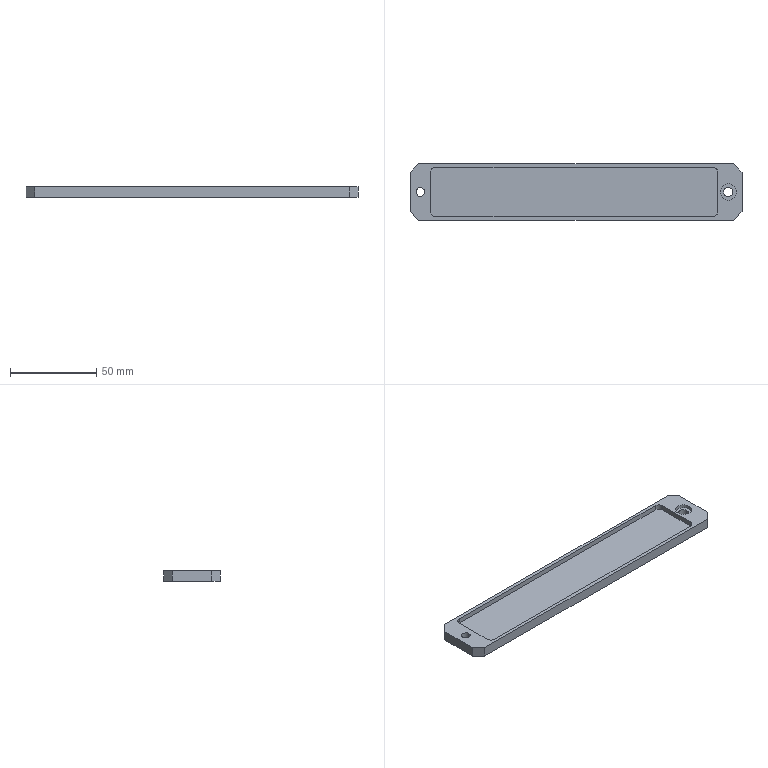Part | STEP file | J454-EBZ05-34-00-Part-1-3 | 1 solid | 26 faces | box 193 x 33 x 6 mm | volume 23054 mm3 | plane 16 | cylinder 10 | commonest cylinder face diameters 6 x4 5 x2 5.5 x2 9.5 x2
STEP:
#1=CARTESIAN_POINT('',(181.75,0.,0.));
#2=VERTEX_POINT('',#1);
#3=CARTESIAN_POINT('',(176.25,0.,0.));
#4=VERTEX_POINT('',#3);
#5=CARTESIAN_POINT('',(179.,0.,0.));
#6=DIRECTION('',(0.,0.,1.));
#7=DIRECTION('',(-1.,0.,0.));
#8=AXIS2_PLACEMENT_3D('',#5,#6,#7);
#9=CIRCLE('',#8,2.75);
#10=EDGE_CURVE('',#2,#4,#9,.T.);
#11=ORIENTED_EDGE('',*,*,#10,.F.);
#12=CARTESIAN_POINT('',(181.75,0.,4.));
#13=VERTEX_POINT('',#12);
#14=CARTESIAN_POINT('',(181.75,0.,6.));
#15=DIRECTION('',(0.,0.,1.));
#16=VECTOR('',#15,1000.);
#17=LINE('',#14,#16);
#18=EDGE_CURVE('',#2,#13,#17,.T.);
#19=ORIENTED_EDGE('',*,*,#18,.T.);
#20=CARTESIAN_POINT('',(176.25,0.,4.));
#21=VERTEX_POINT('',#20);
#22=CARTESIAN_POINT('',(179.,0.,4.));
#23=DIRECTION('',(0.,0.,1.));
#24=DIRECTION('',(-1.,0.,0.));
#25=AXIS2_PLACEMENT_3D('',#22,#23,#24);
#26=CIRCLE('',#25,2.75);
#27=EDGE_CURVE('',#13,#21,#26,.T.);
#28=ORIENTED_EDGE('',*,*,#27,.T.);
#29=CARTESIAN_POINT('',(176.25,0.,6.));
#30=DIRECTION('',(0.,0.,1.));
#31=VECTOR('',#30,1000.);
#32=LINE('',#29,#31);
#33=EDGE_CURVE('',#4,#21,#32,.T.);
#34=ORIENTED_EDGE('',*,*,#33,.F.);
#35=EDGE_LOOP('',(#11,#19,#28,#34));
#36=FACE_OUTER_BOUND('',#35,.T.);
#37=CARTESIAN_POINT('',(179.,0.,6.));
#38=DIRECTION('',(0.,0.,1.));
#39=DIRECTION('',(-1.,0.,0.));
#40=AXIS2_PLACEMENT_3D('',#37,#38,#39);
#41=CYLINDRICAL_SURFACE('',#40,2.75);
#42=ADVANCED_FACE('',(#36),#41,.F.);
#43=CARTESIAN_POINT('',(183.75,0.,4.));
#44=VERTEX_POINT('',#43);
#45=CARTESIAN_POINT('',(174.25,0.,4.));
#46=VERTEX_POINT('',#45);
#47=CARTESIAN_POINT('',(179.,0.,4.));
#48=DIRECTION('',(0.,0.,1.));
#49=DIRECTION('',(-1.,0.,0.));
#50=AXIS2_PLACEMENT_3D('',#47,#48,#49);
#51=CIRCLE('',#50,4.75);
#52=EDGE_CURVE('',#44,#46,#51,.T.);
#53=ORIENTED_EDGE('',*,*,#52,.F.);
#54=CARTESIAN_POINT('',(183.75,0.,6.));
#55=VERTEX_POINT('',#54);
#56=CARTESIAN_POINT('',(183.75,0.,6.));
#57=DIRECTION('',(0.,0.,1.));
#58=VECTOR('',#57,1000.);
#59=LINE('',#56,#58);
#60=EDGE_CURVE('',#44,#55,#59,.T.);
#61=ORIENTED_EDGE('',*,*,#60,.T.);
#62=CARTESIAN_POINT('',(174.25,0.,6.));
#63=VERTEX_POINT('',#62);
#64=CARTESIAN_POINT('',(179.,0.,6.));
#65=DIRECTION('',(0.,0.,1.));
#66=DIRECTION('',(-1.,0.,0.));
#67=AXIS2_PLACEMENT_3D('',#64,#65,#66);
#68=CIRCLE('',#67,4.75);
#69=EDGE_CURVE('',#55,#63,#68,.T.);
#70=ORIENTED_EDGE('',*,*,#69,.T.);
#71=CARTESIAN_POINT('',(174.25,0.,6.));
#72=DIRECTION('',(0.,0.,1.));
#73=VECTOR('',#72,1000.);
#74=LINE('',#71,#73);
#75=EDGE_CURVE('',#46,#63,#74,.T.);
#76=ORIENTED_EDGE('',*,*,#75,.F.);
#77=EDGE_LOOP('',(#53,#61,#70,#76));
#78=FACE_OUTER_BOUND('',#77,.T.);
#79=CARTESIAN_POINT('',(179.,0.,6.));
#80=DIRECTION('',(0.,0.,1.));
#81=DIRECTION('',(-1.,0.,0.));
#82=AXIS2_PLACEMENT_3D('',#79,#80,#81);
#83=CYLINDRICAL_SURFACE('',#82,4.75);
#84=ADVANCED_FACE('',(#78),#83,.F.);
#85=CARTESIAN_POINT('',(2.5,0.,0.));
#86=VERTEX_POINT('',#85);
#87=CARTESIAN_POINT('',(-2.5,0.,0.));
#88=VERTEX_POINT('',#87);
#89=CARTESIAN_POINT('',(0.,0.,0.));
#90=DIRECTION('',(0.,0.,1.));
#91=DIRECTION('',(-1.,0.,0.));
#92=AXIS2_PLACEMENT_3D('',#89,#90,#91);
#93=CIRCLE('',#92,2.5);
#94=EDGE_CURVE('',#86,#88,#93,.T.);
#95=ORIENTED_EDGE('',*,*,#94,.F.);
#96=CARTESIAN_POINT('',(2.5,0.,6.));
#97=VERTEX_POINT('',#96);
#98=CARTESIAN_POINT('',(2.5,0.,0.));
#99=DIRECTION('',(0.,0.,1.));
#100=VECTOR('',#99,1000.);
#101=LINE('',#98,#100);
#102=EDGE_CURVE('',#86,#97,#101,.T.);
#103=ORIENTED_EDGE('',*,*,#102,.T.);
#104=CARTESIAN_POINT('',(-2.5,0.,6.));
#105=VERTEX_POINT('',#104);
#106=CARTESIAN_POINT('',(0.,0.,6.));
#107=DIRECTION('',(0.,0.,-1.));
#108=DIRECTION('',(1.,0.,0.));
#109=AXIS2_PLACEMENT_3D('',#106,#107,#108);
#110=CIRCLE('',#109,2.5);
#111=EDGE_CURVE('',#105,#97,#110,.T.);
#112=ORIENTED_EDGE('',*,*,#111,.F.);
#113=CARTESIAN_POINT('',(-2.5,0.,0.));
#114=DIRECTION('',(0.,0.,1.));
#115=VECTOR('',#114,1000.);
#116=LINE('',#113,#115);
#117=EDGE_CURVE('',#88,#105,#116,.T.);
#118=ORIENTED_EDGE('',*,*,#117,.F.);
#119=EDGE_LOOP('',(#95,#103,#112,#118));
#120=FACE_OUTER_BOUND('',#119,.T.);
#121=CARTESIAN_POINT('',(0.,0.,0.));
#122=DIRECTION('',(0.,0.,1.));
#123=DIRECTION('',(-1.,0.,0.));
#124=AXIS2_PLACEMENT_3D('',#121,#122,#123);
#125=CYLINDRICAL_SURFACE('',#124,2.5);
#126=ADVANCED_FACE('',(#120),#125,.F.);
#127=CARTESIAN_POINT('',(179.,0.,6.));
#128=DIRECTION('',(0.,0.,1.));
#129=DIRECTION('',(-1.,0.,0.));
#130=AXIS2_PLACEMENT_3D('',#127,#128,#129);
#131=CIRCLE('',#130,4.75);
#132=EDGE_CURVE('',#63,#55,#131,.T.);
#133=ORIENTED_EDGE('',*,*,#132,.F.);
#134=ORIENTED_EDGE('',*,*,#69,.F.);
#135=EDGE_LOOP('',(#133,#134));
#136=FACE_BOUND('',#135,.T.);
#137=ORIENTED_EDGE('',*,*,#111,.T.);
#138=CARTESIAN_POINT('',(0.,0.,6.));
#139=DIRECTION('',(0.,0.,-1.));
#140=DIRECTION('',(1.,0.,0.));
#141=AXIS2_PLACEMENT_3D('',#138,#139,#140);
#142=CIRCLE('',#141,2.5);
#143=EDGE_CURVE('',#97,#105,#142,.T.);
#144=ORIENTED_EDGE('',*,*,#143,.T.);
#145=EDGE_LOOP('',(#137,#144));
#146=FACE_BOUND('',#145,.T.);
#147=CARTESIAN_POINT('',(187.,11.5,6.));
#148=VERTEX_POINT('',#147);
#149=CARTESIAN_POINT('',(182.,16.5,6.));
#150=VERTEX_POINT('',#149);
#151=CARTESIAN_POINT('',(144.5,54.,6.));
#152=DIRECTION('',(-0.7071,0.7071,0.));
#153=VECTOR('',#152,1000.);
#154=LINE('',#151,#153);
#155=EDGE_CURVE('',#148,#150,#154,.T.);
#156=ORIENTED_EDGE('',*,*,#155,.T.);
#157=CARTESIAN_POINT('',(-1.,16.5,6.));
#158=VERTEX_POINT('',#157);
#159=CARTESIAN_POINT('',(90.5,16.5,6.));
#160=DIRECTION('',(1.,0.,0.));
#161=VECTOR('',#160,1000.);
#162=LINE('',#159,#161);
#163=EDGE_CURVE('',#158,#150,#162,.T.);
#164=ORIENTED_EDGE('',*,*,#163,.F.);
#165=CARTESIAN_POINT('',(-6.,11.5,6.));
#166=VERTEX_POINT('',#165);
#167=CARTESIAN_POINT('',(36.5,54.,6.));
#168=DIRECTION('',(-0.7071,-0.7071,0.));
#169=VECTOR('',#168,1000.);
#170=LINE('',#167,#169);
#171=EDGE_CURVE('',#158,#166,#170,.T.);
#172=ORIENTED_EDGE('',*,*,#171,.T.);
#173=CARTESIAN_POINT('',(-6.,-11.5,6.));
#174=VERTEX_POINT('',#173);
#175=CARTESIAN_POINT('',(-6.,0.,6.));
#176=DIRECTION('',(0.,1.,0.));
#177=VECTOR('',#176,1000.);
#178=LINE('',#175,#177);
#179=EDGE_CURVE('',#174,#166,#178,.T.);
#180=ORIENTED_EDGE('',*,*,#179,.F.);
#181=CARTESIAN_POINT('',(-1.,-16.5,6.));
#182=VERTEX_POINT('',#181);
#183=CARTESIAN_POINT('',(36.5,-54.,6.));
#184=DIRECTION('',(0.7071,-0.7071,0.));
#185=VECTOR('',#184,1000.);
#186=LINE('',#183,#185);
#187=EDGE_CURVE('',#174,#182,#186,.T.);
#188=ORIENTED_EDGE('',*,*,#187,.T.);
#189=CARTESIAN_POINT('',(182.,-16.5,6.));
#190=VERTEX_POINT('',#189);
#191=CARTESIAN_POINT('',(90.5,-16.5,6.));
#192=DIRECTION('',(-1.,0.,0.));
#193=VECTOR('',#192,1000.);
#194=LINE('',#191,#193);
#195=EDGE_CURVE('',#190,#182,#194,.T.);
#196=ORIENTED_EDGE('',*,*,#195,.F.);
#197=CARTESIAN_POINT('',(187.,-11.5,6.));
#198=VERTEX_POINT('',#197);
#199=CARTESIAN_POINT('',(144.5,-54.,6.));
#200=DIRECTION('',(0.7071,0.7071,0.));
#201=VECTOR('',#200,1000.);
#202=LINE('',#199,#201);
#203=EDGE_CURVE('',#190,#198,#202,.T.);
#204=ORIENTED_EDGE('',*,*,#203,.T.);
#205=CARTESIAN_POINT('',(187.,0.,6.));
#206=DIRECTION('',(0.,-1.,0.));
#207=VECTOR('',#206,1000.);
#208=LINE('',#205,#207);
#209=EDGE_CURVE('',#148,#198,#208,.T.);
#210=ORIENTED_EDGE('',*,*,#209,.F.);
#211=EDGE_LOOP('',(#156,#164,#172,#180,#188,#196,#204,#210));
#212=FACE_OUTER_BOUND('',#211,.T.);
#213=CARTESIAN_POINT('',(170.,14.5,6.));
#214=VERTEX_POINT('',#213);
#215=CARTESIAN_POINT('',(9.,14.5,6.));
#216=VERTEX_POINT('',#215);
#217=CARTESIAN_POINT('',(90.5,14.5,6.));
#218=DIRECTION('',(-1.,0.,0.));
#219=VECTOR('',#218,1000.);
#220=LINE('',#217,#219);
#221=EDGE_CURVE('',#214,#216,#220,.T.);
#222=ORIENTED_EDGE('',*,*,#221,.F.);
#223=CARTESIAN_POINT('',(173.,11.5,6.));
#224=VERTEX_POINT('',#223);
#225=CARTESIAN_POINT('',(170.,11.5,6.));
#226=DIRECTION('',(0.,0.,-1.));
#227=DIRECTION('',(-1.,0.,0.));
#228=AXIS2_PLACEMENT_3D('',#225,#226,#227);
#229=CIRCLE('',#228,3.);
#230=EDGE_CURVE('',#214,#224,#229,.T.);
#231=ORIENTED_EDGE('',*,*,#230,.T.);
#232=CARTESIAN_POINT('',(173.,-11.5,6.));
#233=VERTEX_POINT('',#232);
#234=CARTESIAN_POINT('',(173.,0.,6.));
#235=DIRECTION('',(0.,1.,0.));
#236=VECTOR('',#235,1000.);
#237=LINE('',#234,#236);
#238=EDGE_CURVE('',#233,#224,#237,.T.);
#239=ORIENTED_EDGE('',*,*,#238,.F.);
#240=CARTESIAN_POINT('',(170.,-14.5,6.));
#241=VERTEX_POINT('',#240);
#242=CARTESIAN_POINT('',(170.,-11.5,6.));
#243=DIRECTION('',(0.,0.,-1.));
#244=DIRECTION('',(-1.,0.,0.));
#245=AXIS2_PLACEMENT_3D('',#242,#243,#244);
#246=CIRCLE('',#245,3.);
#247=EDGE_CURVE('',#233,#241,#246,.T.);
#248=ORIENTED_EDGE('',*,*,#247,.T.);
#249=CARTESIAN_POINT('',(9.,-14.5,6.));
#250=VERTEX_POINT('',#249);
#251=CARTESIAN_POINT('',(90.5,-14.5,6.));
#252=DIRECTION('',(1.,0.,0.));
#253=VECTOR('',#252,1000.);
#254=LINE('',#251,#253);
#255=EDGE_CURVE('',#250,#241,#254,.T.);
#256=ORIENTED_EDGE('',*,*,#255,.F.);
#257=CARTESIAN_POINT('',(6.,-11.5,6.));
#258=VERTEX_POINT('',#257);
#259=CARTESIAN_POINT('',(9.,-11.5,6.));
#260=DIRECTION('',(0.,0.,-1.));
#261=DIRECTION('',(-1.,0.,0.));
#262=AXIS2_PLACEMENT_3D('',#259,#260,#261);
#263=CIRCLE('',#262,3.);
#264=EDGE_CURVE('',#250,#258,#263,.T.);
#265=ORIENTED_EDGE('',*,*,#264,.T.);
#266=CARTESIAN_POINT('',(6.,11.5,6.));
#267=VERTEX_POINT('',#266);
#268=CARTESIAN_POINT('',(6.,0.,6.));
#269=DIRECTION('',(0.,-1.,0.));
#270=VECTOR('',#269,1000.);
#271=LINE('',#268,#270);
#272=EDGE_CURVE('',#267,#258,#271,.T.);
#273=ORIENTED_EDGE('',*,*,#272,.F.);
#274=CARTESIAN_POINT('',(9.,11.5,6.));
#275=DIRECTION('',(0.,0.,-1.));
#276=DIRECTION('',(-1.,0.,0.));
#277=AXIS2_PLACEMENT_3D('',#274,#275,#276);
#278=CIRCLE('',#277,3.);
#279=EDGE_CURVE('',#267,#216,#278,.T.);
#280=ORIENTED_EDGE('',*,*,#279,.T.);
#281=EDGE_LOOP('',(#222,#231,#239,#248,#256,#265,#273,#280));
#282=FACE_BOUND('',#281,.T.);
#283=CARTESIAN_POINT('',(90.5,0.,6.));
#284=DIRECTION('',(0.,0.,1.));
#285=DIRECTION('',(-1.,0.,0.));
#286=AXIS2_PLACEMENT_3D('',#283,#284,#285);
#287=PLANE('',#286);
#288=ADVANCED_FACE('',(#136,#146,#212,#282),#287,.T.);
#289=CARTESIAN_POINT('',(182.,16.5,0.));
#290=VERTEX_POINT('',#289);
#291=CARTESIAN_POINT('',(-1.,16.5,0.));
#292=VERTEX_POINT('',#291);
#293=CARTESIAN_POINT('',(90.5,16.5,0.));
#294=DIRECTION('',(-1.,0.,0.));
#295=VECTOR('',#294,1000.);
#296=LINE('',#293,#295);
#297=EDGE_CURVE('',#290,#292,#296,.T.);
#298=ORIENTED_EDGE('',*,*,#297,.T.);
#299=CARTESIAN_POINT('',(-1.,16.5,0.));
#300=DIRECTION('',(0.,0.,1.));
#301=VECTOR('',#300,1000.);
#302=LINE('',#299,#301);
#303=EDGE_CURVE('',#292,#158,#302,.T.);
#304=ORIENTED_EDGE('',*,*,#303,.T.);
#305=ORIENTED_EDGE('',*,*,#163,.T.);
#306=CARTESIAN_POINT('',(182.,16.5,0.));
#307=DIRECTION('',(0.,0.,-1.));
#308=VECTOR('',#307,1000.);
#309=LINE('',#306,#308);
#310=EDGE_CURVE('',#150,#290,#309,.T.);
#311=ORIENTED_EDGE('',*,*,#310,.T.);
#312=EDGE_LOOP('',(#298,#304,#305,#311));
#313=FACE_OUTER_BOUND('',#312,.T.);
#314=CARTESIAN_POINT('',(90.5,16.5,0.));
#315=DIRECTION('',(0.,1.,0.));
#316=DIRECTION('',(0.,0.,-1.));
#317=AXIS2_PLACEMENT_3D('',#314,#315,#316);
#318=PLANE('',#317);
#319=ADVANCED_FACE('',(#313),#318,.T.);
#320=CARTESIAN_POINT('',(187.,-11.5,0.));
#321=VERTEX_POINT('',#320);
#322=CARTESIAN_POINT('',(187.,11.5,0.));
#323=VERTEX_POINT('',#322);
#324=CARTESIAN_POINT('',(187.,0.,0.));
#325=DIRECTION('',(0.,1.,0.));
#326=VECTOR('',#325,1000.);
#327=LINE('',#324,#326);
#328=EDGE_CURVE('',#321,#323,#327,.T.);
#329=ORIENTED_EDGE('',*,*,#328,.T.);
#330=CARTESIAN_POINT('',(187.,11.5,0.));
#331=DIRECTION('',(0.,0.,1.));
#332=VECTOR('',#331,1000.);
#333=LINE('',#330,#332);
#334=EDGE_CURVE('',#323,#148,#333,.T.);
#335=ORIENTED_EDGE('',*,*,#334,.T.);
#336=ORIENTED_EDGE('',*,*,#209,.T.);
#337=CARTESIAN_POINT('',(187.,-11.5,0.));
#338=DIRECTION('',(0.,0.,-1.));
#339=VECTOR('',#338,1000.);
#340=LINE('',#337,#339);
#341=EDGE_CURVE('',#198,#321,#340,.T.);
#342=ORIENTED_EDGE('',*,*,#341,.T.);
#343=EDGE_LOOP('',(#329,#335,#336,#342));
#344=FACE_OUTER_BOUND('',#343,.T.);
#345=CARTESIAN_POINT('',(187.,0.,0.));
#346=DIRECTION('',(1.,0.,0.));
#347=DIRECTION('',(0.,0.,1.));
#348=AXIS2_PLACEMENT_3D('',#345,#346,#347);
#349=PLANE('',#348);
#350=ADVANCED_FACE('',(#344),#349,.T.);
#351=ORIENTED_EDGE('',*,*,#195,.T.);
#352=CARTESIAN_POINT('',(-1.,-16.5,0.));
#353=VERTEX_POINT('',#352);
#354=CARTESIAN_POINT('',(-1.,-16.5,0.));
#355=DIRECTION('',(0.,0.,-1.));
#356=VECTOR('',#355,1000.);
#357=LINE('',#354,#356);
#358=EDGE_CURVE('',#182,#353,#357,.T.);
#359=ORIENTED_EDGE('',*,*,#358,.T.);
#360=CARTESIAN_POINT('',(182.,-16.5,0.));
#361=VERTEX_POINT('',#360);
#362=CARTESIAN_POINT('',(90.5,-16.5,0.));
#363=DIRECTION('',(1.,0.,0.));
#364=VECTOR('',#363,1000.);
#365=LINE('',#362,#364);
#366=EDGE_CURVE('',#353,#361,#365,.T.);
#367=ORIENTED_EDGE('',*,*,#366,.T.);
#368=CARTESIAN_POINT('',(182.,-16.5,0.));
#369=DIRECTION('',(0.,0.,1.));
#370=VECTOR('',#369,1000.);
#371=LINE('',#368,#370);
#372=EDGE_CURVE('',#361,#190,#371,.T.);
#373=ORIENTED_EDGE('',*,*,#372,.T.);
#374=EDGE_LOOP('',(#351,#359,#367,#373));
#375=FACE_OUTER_BOUND('',#374,.T.);
#376=CARTESIAN_POINT('',(90.5,-16.5,0.));
#377=DIRECTION('',(0.,-1.,0.));
#378=DIRECTION('',(0.,0.,1.));
#379=AXIS2_PLACEMENT_3D('',#376,#377,#378);
#380=PLANE('',#379);
#381=ADVANCED_FACE('',(#375),#380,.T.);
#382=CARTESIAN_POINT('',(179.,0.,0.));
#383=DIRECTION('',(0.,0.,1.));
#384=DIRECTION('',(-1.,0.,0.));
#385=AXIS2_PLACEMENT_3D('',#382,#383,#384);
#386=CIRCLE('',#385,2.75);
#387=EDGE_CURVE('',#4,#2,#386,.T.);
#388=ORIENTED_EDGE('',*,*,#387,.T.);
#389=ORIENTED_EDGE('',*,*,#10,.T.);
#390=EDGE_LOOP('',(#388,#389));
#391=FACE_BOUND('',#390,.T.);
#392=CARTESIAN_POINT('',(0.,0.,0.));
#393=DIRECTION('',(0.,0.,1.));
#394=DIRECTION('',(-1.,0.,0.));
#395=AXIS2_PLACEMENT_3D('',#392,#393,#394);
#396=CIRCLE('',#395,2.5);
#397=EDGE_CURVE('',#88,#86,#396,.T.);
#398=ORIENTED_EDGE('',*,*,#397,.T.);
#399=ORIENTED_EDGE('',*,*,#94,.T.);
#400=EDGE_LOOP('',(#398,#399));
#401=FACE_BOUND('',#400,.T.);
#402=CARTESIAN_POINT('',(-6.,11.5,0.));
#403=VERTEX_POINT('',#402);
#404=CARTESIAN_POINT('',(-6.,-11.5,0.));
#405=VERTEX_POINT('',#404);
#406=CARTESIAN_POINT('',(-6.,0.,0.));
#407=DIRECTION('',(0.,-1.,0.));
#408=VECTOR('',#407,1000.);
#409=LINE('',#406,#408);
#410=EDGE_CURVE('',#403,#405,#409,.T.);
#411=ORIENTED_EDGE('',*,*,#410,.F.);
#412=CARTESIAN_POINT('',(36.5,54.,0.));
#413=DIRECTION('',(0.7071,0.7071,0.));
#414=VECTOR('',#413,1000.);
#415=LINE('',#412,#414);
#416=EDGE_CURVE('',#403,#292,#415,.T.);
#417=ORIENTED_EDGE('',*,*,#416,.T.);
#418=ORIENTED_EDGE('',*,*,#297,.F.);
#419=CARTESIAN_POINT('',(144.5,54.,0.));
#420=DIRECTION('',(0.7071,-0.7071,0.));
#421=VECTOR('',#420,1000.);
#422=LINE('',#419,#421);
#423=EDGE_CURVE('',#290,#323,#422,.T.);
#424=ORIENTED_EDGE('',*,*,#423,.T.);
#425=ORIENTED_EDGE('',*,*,#328,.F.);
#426=CARTESIAN_POINT('',(144.5,-54.,0.));
#427=DIRECTION('',(-0.7071,-0.7071,0.));
#428=VECTOR('',#427,1000.);
#429=LINE('',#426,#428);
#430=EDGE_CURVE('',#321,#361,#429,.T.);
#431=ORIENTED_EDGE('',*,*,#430,.T.);
#432=ORIENTED_EDGE('',*,*,#366,.F.);
#433=CARTESIAN_POINT('',(36.5,-54.,0.));
#434=DIRECTION('',(-0.7071,0.7071,0.));
#435=VECTOR('',#434,1000.);
#436=LINE('',#433,#435);
#437=EDGE_CURVE('',#353,#405,#436,.T.);
#438=ORIENTED_EDGE('',*,*,#437,.T.);
#439=EDGE_LOOP('',(#411,#417,#418,#424,#425,#431,#432,#438));
#440=FACE_OUTER_BOUND('',#439,.T.);
#441=CARTESIAN_POINT('',(90.5,0.,0.));
#442=DIRECTION('',(0.,0.,-1.));
#443=DIRECTION('',(1.,0.,0.));
#444=AXIS2_PLACEMENT_3D('',#441,#442,#443);
#445=PLANE('',#444);
#446=ADVANCED_FACE('',(#391,#401,#440),#445,.T.);
#447=ORIENTED_EDGE('',*,*,#179,.T.);
#448=CARTESIAN_POINT('',(-6.,11.5,0.));
#449=DIRECTION('',(0.,0.,-1.));
#450=VECTOR('',#449,1000.);
#451=LINE('',#448,#450);
#452=EDGE_CURVE('',#166,#403,#451,.T.);
#453=ORIENTED_EDGE('',*,*,#452,.T.);
#454=ORIENTED_EDGE('',*,*,#410,.T.);
#455=CARTESIAN_POINT('',(-6.,-11.5,0.));
#456=DIRECTION('',(0.,0.,1.));
#457=VECTOR('',#456,1000.);
#458=LINE('',#455,#457);
#459=EDGE_CURVE('',#405,#174,#458,.T.);
#460=ORIENTED_EDGE('',*,*,#459,.T.);
#461=EDGE_LOOP('',(#447,#453,#454,#460));
#462=FACE_OUTER_BOUND('',#461,.T.);
#463=CARTESIAN_POINT('',(-6.,0.,0.));
#464=DIRECTION('',(-1.,0.,0.));
#465=DIRECTION('',(0.,0.,-1.));
#466=AXIS2_PLACEMENT_3D('',#463,#464,#465);
#467=PLANE('',#466);
#468=ADVANCED_FACE('',(#462),#467,.T.);
#469=CARTESIAN_POINT('',(170.,14.5,3.));
#470=VERTEX_POINT('',#469);
#471=CARTESIAN_POINT('',(9.,14.5,3.));
#472=VERTEX_POINT('',#471);
#473=CARTESIAN_POINT('',(89.5,14.5,3.));
#474=DIRECTION('',(-1.,0.,0.));
#475=VECTOR('',#474,1000.);
#476=LINE('',#473,#475);
#477=EDGE_CURVE('',#470,#472,#476,.T.);
#478=ORIENTED_EDGE('',*,*,#477,.F.);
#479=CARTESIAN_POINT('',(170.,14.5,6.));
#480=DIRECTION('',(0.,0.,1.));
#481=VECTOR('',#480,1000.);
#482=LINE('',#479,#481);
#483=EDGE_CURVE('',#470,#214,#482,.T.);
#484=ORIENTED_EDGE('',*,*,#483,.T.);
#485=ORIENTED_EDGE('',*,*,#221,.T.);
#486=CARTESIAN_POINT('',(9.,14.5,3.));
#487=DIRECTION('',(0.,0.,-1.));
#488=VECTOR('',#487,1000.);
#489=LINE('',#486,#488);
#490=EDGE_CURVE('',#216,#472,#489,.T.);
#491=ORIENTED_EDGE('',*,*,#490,.T.);
#492=EDGE_LOOP('',(#478,#484,#485,#491));
#493=FACE_OUTER_BOUND('',#492,.T.);
#494=CARTESIAN_POINT('',(89.5,14.5,3.));
#495=DIRECTION('',(0.,1.,0.));
#496=DIRECTION('',(0.,0.,-1.));
#497=AXIS2_PLACEMENT_3D('',#494,#495,#496);
#498=PLANE('',#497);
#499=ADVANCED_FACE('',(#493),#498,.F.);
#500=CARTESIAN_POINT('',(173.,-11.5,3.));
#501=VERTEX_POINT('',#500);
#502=CARTESIAN_POINT('',(173.,11.5,3.));
#503=VERTEX_POINT('',#502);
#504=CARTESIAN_POINT('',(173.,0.,3.));
#505=DIRECTION('',(0.,1.,0.));
#506=VECTOR('',#505,1000.);
#507=LINE('',#504,#506);
#508=EDGE_CURVE('',#501,#503,#507,.T.);
#509=ORIENTED_EDGE('',*,*,#508,.F.);
#510=CARTESIAN_POINT('',(173.,-11.5,6.));
#511=DIRECTION('',(0.,0.,1.));
#512=VECTOR('',#511,1000.);
#513=LINE('',#510,#512);
#514=EDGE_CURVE('',#501,#233,#513,.T.);
#515=ORIENTED_EDGE('',*,*,#514,.T.);
#516=ORIENTED_EDGE('',*,*,#238,.T.);
#517=CARTESIAN_POINT('',(173.,11.5,3.));
#518=DIRECTION('',(0.,0.,-1.));
#519=VECTOR('',#518,1000.);
#520=LINE('',#517,#519);
#521=EDGE_CURVE('',#224,#503,#520,.T.);
#522=ORIENTED_EDGE('',*,*,#521,.T.);
#523=EDGE_LOOP('',(#509,#515,#516,#522));
#524=FACE_OUTER_BOUND('',#523,.T.);
#525=CARTESIAN_POINT('',(173.,0.,3.));
#526=DIRECTION('',(1.,0.,0.));
#527=DIRECTION('',(0.,0.,1.));
#528=AXIS2_PLACEMENT_3D('',#525,#526,#527);
#529=PLANE('',#528);
#530=ADVANCED_FACE('',(#524),#529,.F.);
#531=ORIENTED_EDGE('',*,*,#255,.T.);
#532=CARTESIAN_POINT('',(170.,-14.5,3.));
#533=VERTEX_POINT('',#532);
#534=CARTESIAN_POINT('',(170.,-14.5,3.));
#535=DIRECTION('',(0.,0.,-1.));
#536=VECTOR('',#535,1000.);
#537=LINE('',#534,#536);
#538=EDGE_CURVE('',#241,#533,#537,.T.);
#539=ORIENTED_EDGE('',*,*,#538,.T.);
#540=CARTESIAN_POINT('',(9.,-14.5,3.));
#541=VERTEX_POINT('',#540);
#542=CARTESIAN_POINT('',(89.5,-14.5,3.));
#543=DIRECTION('',(1.,0.,0.));
#544=VECTOR('',#543,1000.);
#545=LINE('',#542,#544);
#546=EDGE_CURVE('',#541,#533,#545,.T.);
#547=ORIENTED_EDGE('',*,*,#546,.F.);
#548=CARTESIAN_POINT('',(9.,-14.5,6.));
#549=DIRECTION('',(0.,0.,1.));
#550=VECTOR('',#549,1000.);
#551=LINE('',#548,#550);
#552=EDGE_CURVE('',#541,#250,#551,.T.);
#553=ORIENTED_EDGE('',*,*,#552,.T.);
#554=EDGE_LOOP('',(#531,#539,#547,#553));
#555=FACE_OUTER_BOUND('',#554,.T.);
#556=CARTESIAN_POINT('',(89.5,-14.5,3.));
#557=DIRECTION('',(0.,-1.,0.));
#558=DIRECTION('',(0.,0.,1.));
#559=AXIS2_PLACEMENT_3D('',#556,#557,#558);
#560=PLANE('',#559);
#561=ADVANCED_FACE('',(#555),#560,.F.);
#562=ORIENTED_EDGE('',*,*,#546,.T.);
#563=CARTESIAN_POINT('',(170.,-11.5,3.));
#564=DIRECTION('',(0.,0.,1.));
#565=DIRECTION('',(1.,0.,0.));
#566=AXIS2_PLACEMENT_3D('',#563,#564,#565);
#567=CIRCLE('',#566,3.);
#568=EDGE_CURVE('',#533,#501,#567,.T.);
#569=ORIENTED_EDGE('',*,*,#568,.T.);
#570=ORIENTED_EDGE('',*,*,#508,.T.);
#571=CARTESIAN_POINT('',(170.,11.5,3.));
#572=DIRECTION('',(0.,0.,1.));
#573=DIRECTION('',(1.,0.,0.));
#574=AXIS2_PLACEMENT_3D('',#571,#572,#573);
#575=CIRCLE('',#574,3.);
#576=EDGE_CURVE('',#503,#470,#575,.T.);
#577=ORIENTED_EDGE('',*,*,#576,.T.);
#578=ORIENTED_EDGE('',*,*,#477,.T.);
#579=CARTESIAN_POINT('',(6.,11.5,3.));
#580=VERTEX_POINT('',#579);
#581=CARTESIAN_POINT('',(9.,11.5,3.));
#582=DIRECTION('',(0.,0.,1.));
#583=DIRECTION('',(1.,0.,0.));
#584=AXIS2_PLACEMENT_3D('',#581,#582,#583);
#585=CIRCLE('',#584,3.);
#586=EDGE_CURVE('',#472,#580,#585,.T.);
#587=ORIENTED_EDGE('',*,*,#586,.T.);
#588=CARTESIAN_POINT('',(6.,-11.5,3.));
#589=VERTEX_POINT('',#588);
#590=CARTESIAN_POINT('',(6.,0.,3.));
#591=DIRECTION('',(0.,-1.,0.));
#592=VECTOR('',#591,1000.);
#593=LINE('',#590,#592);
#594=EDGE_CURVE('',#580,#589,#593,.T.);
#595=ORIENTED_EDGE('',*,*,#594,.T.);
#596=CARTESIAN_POINT('',(9.,-11.5,3.));
#597=DIRECTION('',(0.,0.,1.));
#598=DIRECTION('',(1.,0.,0.));
#599=AXIS2_PLACEMENT_3D('',#596,#597,#598);
#600=CIRCLE('',#599,3.);
#601=EDGE_CURVE('',#589,#541,#600,.T.);
#602=ORIENTED_EDGE('',*,*,#601,.T.);
#603=EDGE_LOOP('',(#562,#569,#570,#577,#578,#587,#595,#602));
#604=FACE_OUTER_BOUND('',#603,.T.);
#605=CARTESIAN_POINT('',(89.5,0.,3.));
#606=DIRECTION('',(0.,0.,-1.));
#607=DIRECTION('',(1.,0.,0.));
#608=AXIS2_PLACEMENT_3D('',#605,#606,#607);
#609=PLANE('',#608);
#610=ADVANCED_FACE('',(#604),#609,.F.);
#611=ORIENTED_EDGE('',*,*,#272,.T.);
#612=CARTESIAN_POINT('',(6.,-11.5,3.));
#613=DIRECTION('',(0.,0.,-1.));
#614=VECTOR('',#613,1000.);
#615=LINE('',#612,#614);
#616=EDGE_CURVE('',#258,#589,#615,.T.);
#617=ORIENTED_EDGE('',*,*,#616,.T.);
#618=ORIENTED_EDGE('',*,*,#594,.F.);
#619=CARTESIAN_POINT('',(6.,11.5,6.));
#620=DIRECTION('',(0.,0.,1.));
#621=VECTOR('',#620,1000.);
#622=LINE('',#619,#621);
#623=EDGE_CURVE('',#580,#267,#622,.T.);
#624=ORIENTED_EDGE('',*,*,#623,.T.);
#625=EDGE_LOOP('',(#611,#617,#618,#624));
#626=FACE_OUTER_BOUND('',#625,.T.);
#627=CARTESIAN_POINT('',(6.,0.,3.));
#628=DIRECTION('',(-1.,0.,0.));
#629=DIRECTION('',(0.,0.,-1.));
#630=AXIS2_PLACEMENT_3D('',#627,#628,#629);
#631=PLANE('',#630);
#632=ADVANCED_FACE('',(#626),#631,.F.);
#633=ORIENTED_EDGE('',*,*,#586,.F.);
#634=ORIENTED_EDGE('',*,*,#490,.F.);
#635=ORIENTED_EDGE('',*,*,#279,.F.);
#636=ORIENTED_EDGE('',*,*,#623,.F.);
#637=EDGE_LOOP('',(#633,#634,#635,#636));
#638=FACE_OUTER_BOUND('',#637,.T.);
#639=CARTESIAN_POINT('',(9.,11.5,3.));
#640=DIRECTION('',(0.,0.,-1.));
#641=DIRECTION('',(1.,0.,0.));
#642=AXIS2_PLACEMENT_3D('',#639,#640,#641);
#643=CYLINDRICAL_SURFACE('',#642,3.);
#644=ADVANCED_FACE('',(#638),#643,.F.);
#645=ORIENTED_EDGE('',*,*,#601,.F.);
#646=ORIENTED_EDGE('',*,*,#616,.F.);
#647=ORIENTED_EDGE('',*,*,#264,.F.);
#648=ORIENTED_EDGE('',*,*,#552,.F.);
#649=EDGE_LOOP('',(#645,#646,#647,#648));
#650=FACE_OUTER_BOUND('',#649,.T.);
#651=CARTESIAN_POINT('',(9.,-11.5,3.));
#652=DIRECTION('',(0.,0.,-1.));
#653=DIRECTION('',(1.,0.,0.));
#654=AXIS2_PLACEMENT_3D('',#651,#652,#653);
#655=CYLINDRICAL_SURFACE('',#654,3.);
#656=ADVANCED_FACE('',(#650),#655,.F.);
#657=ORIENTED_EDGE('',*,*,#430,.F.);
#658=ORIENTED_EDGE('',*,*,#341,.F.);
#659=ORIENTED_EDGE('',*,*,#203,.F.);
#660=ORIENTED_EDGE('',*,*,#372,.F.);
#661=EDGE_LOOP('',(#657,#658,#659,#660));
#662=FACE_OUTER_BOUND('',#661,.T.);
#663=CARTESIAN_POINT('',(182.,-16.5,0.));
#664=DIRECTION('',(-0.7071,0.7071,0.));
#665=DIRECTION('',(0.,0.,1.));
#666=AXIS2_PLACEMENT_3D('',#663,#664,#665);
#667=PLANE('',#666);
#668=ADVANCED_FACE('',(#662),#667,.F.);
#669=ORIENTED_EDGE('',*,*,#423,.F.);
#670=ORIENTED_EDGE('',*,*,#310,.F.);
#671=ORIENTED_EDGE('',*,*,#155,.F.);
#672=ORIENTED_EDGE('',*,*,#334,.F.);
#673=EDGE_LOOP('',(#669,#670,#671,#672));
#674=FACE_OUTER_BOUND('',#673,.T.);
#675=CARTESIAN_POINT('',(187.,11.5,0.));
#676=DIRECTION('',(-0.7071,-0.7071,0.));
#677=DIRECTION('',(0.,0.,1.));
#678=AXIS2_PLACEMENT_3D('',#675,#676,#677);
#679=PLANE('',#678);
#680=ADVANCED_FACE('',(#674),#679,.F.);
#681=ORIENTED_EDGE('',*,*,#437,.F.);
#682=ORIENTED_EDGE('',*,*,#358,.F.);
#683=ORIENTED_EDGE('',*,*,#187,.F.);
#684=ORIENTED_EDGE('',*,*,#459,.F.);
#685=EDGE_LOOP('',(#681,#682,#683,#684));
#686=FACE_OUTER_BOUND('',#685,.T.);
#687=CARTESIAN_POINT('',(-6.,-11.5,0.));
#688=DIRECTION('',(0.7071,0.7071,0.));
#689=DIRECTION('',(0.,0.,1.));
#690=AXIS2_PLACEMENT_3D('',#687,#688,#689);
#691=PLANE('',#690);
#692=ADVANCED_FACE('',(#686),#691,.F.);
#693=ORIENTED_EDGE('',*,*,#416,.F.);
#694=ORIENTED_EDGE('',*,*,#452,.F.);
#695=ORIENTED_EDGE('',*,*,#171,.F.);
#696=ORIENTED_EDGE('',*,*,#303,.F.);
#697=EDGE_LOOP('',(#693,#694,#695,#696));
#698=FACE_OUTER_BOUND('',#697,.T.);
#699=CARTESIAN_POINT('',(-1.,16.5,0.));
#700=DIRECTION('',(0.7071,-0.7071,0.));
#701=DIRECTION('',(0.,0.,1.));
#702=AXIS2_PLACEMENT_3D('',#699,#700,#701);
#703=PLANE('',#702);
#704=ADVANCED_FACE('',(#698),#703,.F.);
#705=ORIENTED_EDGE('',*,*,#576,.F.);
#706=ORIENTED_EDGE('',*,*,#521,.F.);
#707=ORIENTED_EDGE('',*,*,#230,.F.);
#708=ORIENTED_EDGE('',*,*,#483,.F.);
#709=EDGE_LOOP('',(#705,#706,#707,#708));
#710=FACE_OUTER_BOUND('',#709,.T.);
#711=CARTESIAN_POINT('',(170.,11.5,3.));
#712=DIRECTION('',(0.,0.,-1.));
#713=DIRECTION('',(1.,0.,0.));
#714=AXIS2_PLACEMENT_3D('',#711,#712,#713);
#715=CYLINDRICAL_SURFACE('',#714,3.);
#716=ADVANCED_FACE('',(#710),#715,.F.);
#717=ORIENTED_EDGE('',*,*,#568,.F.);
#718=ORIENTED_EDGE('',*,*,#538,.F.);
#719=ORIENTED_EDGE('',*,*,#247,.F.);
#720=ORIENTED_EDGE('',*,*,#514,.F.);
#721=EDGE_LOOP('',(#717,#718,#719,#720));
#722=FACE_OUTER_BOUND('',#721,.T.);
#723=CARTESIAN_POINT('',(170.,-11.5,3.));
#724=DIRECTION('',(0.,0.,-1.));
#725=DIRECTION('',(1.,0.,0.));
#726=AXIS2_PLACEMENT_3D('',#723,#724,#725);
#727=CYLINDRICAL_SURFACE('',#726,3.);
#728=ADVANCED_FACE('',(#722),#727,.F.);
#729=ORIENTED_EDGE('',*,*,#102,.F.);
#730=ORIENTED_EDGE('',*,*,#397,.F.);
#731=ORIENTED_EDGE('',*,*,#117,.T.);
#732=ORIENTED_EDGE('',*,*,#143,.F.);
#733=EDGE_LOOP('',(#729,#730,#731,#732));
#734=FACE_OUTER_BOUND('',#733,.T.);
#735=CARTESIAN_POINT('',(0.,0.,0.));
#736=DIRECTION('',(0.,0.,1.));
#737=DIRECTION('',(-1.,0.,0.));
#738=AXIS2_PLACEMENT_3D('',#735,#736,#737);
#739=CYLINDRICAL_SURFACE('',#738,2.5);
#740=ADVANCED_FACE('',(#734),#739,.F.);
#741=ORIENTED_EDGE('',*,*,#60,.F.);
#742=CARTESIAN_POINT('',(179.,0.,4.));
#743=DIRECTION('',(0.,0.,1.));
#744=DIRECTION('',(-1.,0.,0.));
#745=AXIS2_PLACEMENT_3D('',#742,#743,#744);
#746=CIRCLE('',#745,4.75);
#747=EDGE_CURVE('',#46,#44,#746,.T.);
#748=ORIENTED_EDGE('',*,*,#747,.F.);
#749=ORIENTED_EDGE('',*,*,#75,.T.);
#750=ORIENTED_EDGE('',*,*,#132,.T.);
#751=EDGE_LOOP('',(#741,#748,#749,#750));
#752=FACE_OUTER_BOUND('',#751,.T.);
#753=CARTESIAN_POINT('',(179.,0.,6.));
#754=DIRECTION('',(0.,0.,1.));
#755=DIRECTION('',(-1.,0.,0.));
#756=AXIS2_PLACEMENT_3D('',#753,#754,#755);
#757=CYLINDRICAL_SURFACE('',#756,4.75);
#758=ADVANCED_FACE('',(#752),#757,.F.);
#759=CARTESIAN_POINT('',(179.,0.,4.));
#760=DIRECTION('',(0.,0.,1.));
#761=DIRECTION('',(-1.,0.,0.));
#762=AXIS2_PLACEMENT_3D('',#759,#760,#761);
#763=CIRCLE('',#762,2.75);
#764=EDGE_CURVE('',#21,#13,#763,.T.);
#765=ORIENTED_EDGE('',*,*,#764,.F.);
#766=ORIENTED_EDGE('',*,*,#27,.F.);
#767=EDGE_LOOP('',(#765,#766));
#768=FACE_BOUND('',#767,.T.);
#769=ORIENTED_EDGE('',*,*,#747,.T.);
#770=ORIENTED_EDGE('',*,*,#52,.T.);
#771=EDGE_LOOP('',(#769,#770));
#772=FACE_OUTER_BOUND('',#771,.T.);
#773=CARTESIAN_POINT('',(183.75,0.,4.));
#774=DIRECTION('',(0.,0.,-1.));
#775=DIRECTION('',(1.,0.,0.));
#776=AXIS2_PLACEMENT_3D('',#773,#774,#775);
#777=PLANE('',#776);
#778=ADVANCED_FACE('',(#768,#772),#777,.F.);
#779=ORIENTED_EDGE('',*,*,#18,.F.);
#780=ORIENTED_EDGE('',*,*,#387,.F.);
#781=ORIENTED_EDGE('',*,*,#33,.T.);
#782=ORIENTED_EDGE('',*,*,#764,.T.);
#783=EDGE_LOOP('',(#779,#780,#781,#782));
#784=FACE_OUTER_BOUND('',#783,.T.);
#785=CARTESIAN_POINT('',(179.,0.,6.));
#786=DIRECTION('',(0.,0.,1.));
#787=DIRECTION('',(-1.,0.,0.));
#788=AXIS2_PLACEMENT_3D('',#785,#786,#787);
#789=CYLINDRICAL_SURFACE('',#788,2.75);
#790=ADVANCED_FACE('',(#784),#789,.F.);
#791=CLOSED_SHELL('',(#42,#84,#126,#288,#319,#350,#381,#446,#468,#499,#530,#561,#610,#632,#644,#656,#668,#680,#692,#704,#716,#728,#740,#758,#778,#790));
#792=MANIFOLD_SOLID_BREP('',#791);
#793=CARTESIAN_POINT('',(0.,0.,0.));
#794=DIRECTION('',(0.,0.,1.));
#795=DIRECTION('',(1.,0.,0.));
#796=AXIS2_PLACEMENT_3D('',#793,#794,#795);
#797=(LENGTH_UNIT()NAMED_UNIT(*)SI_UNIT(.MILLI.,.METRE.));
#798=UNCERTAINTY_MEASURE_WITH_UNIT(LENGTH_MEASURE(0.00001),#797,'','');
#799=(NAMED_UNIT(*)PLANE_ANGLE_UNIT()SI_UNIT($,.RADIAN.));
#800=(NAMED_UNIT(*)SI_UNIT($,.STERADIAN.)SOLID_ANGLE_UNIT());
#801=(GEOMETRIC_REPRESENTATION_CONTEXT(3)GLOBAL_UNCERTAINTY_ASSIGNED_CONTEXT((#798))GLOBAL_UNIT_ASSIGNED_CONTEXT((#797,#799,#800))REPRESENTATION_CONTEXT('',''));
#802=ADVANCED_BREP_SHAPE_REPRESENTATION('',(#792,#796),#801);